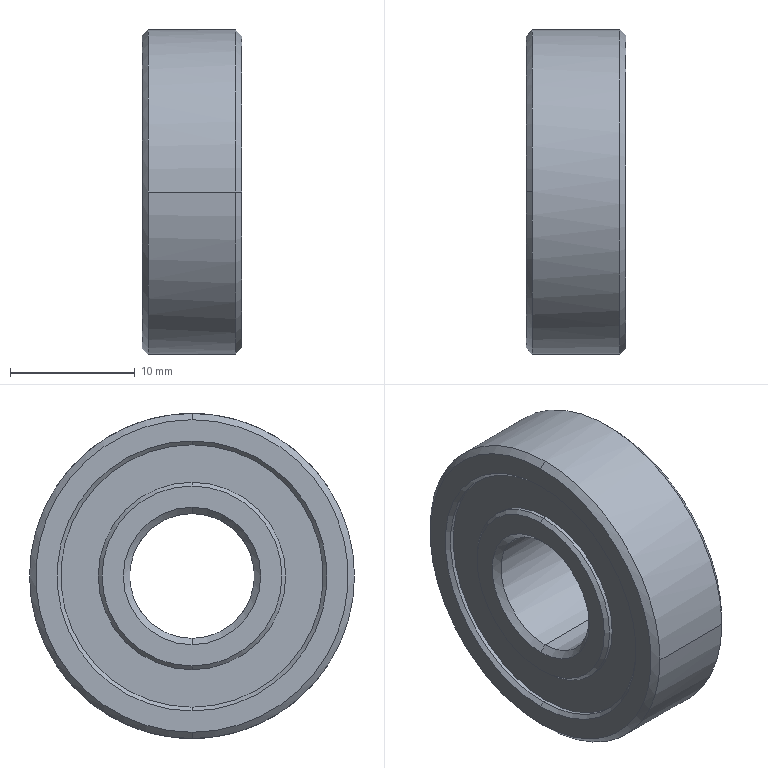Part | STEP file | 6000ZZ-1 | 1 solid | 34 faces | box 8 x 26 x 26 mm | volume 3377 mm3 | cone 16 | cylinder 12 | plane 6 | commonest cylinder face diameters 15 x4 21 x4 10 x2 26 x2